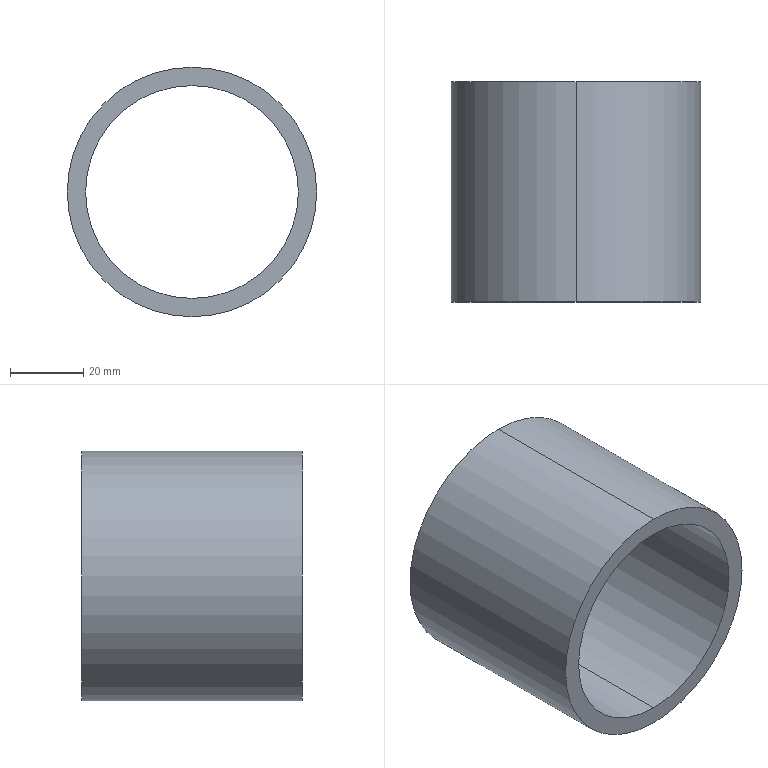Part | STEP file | outer cylinder block | 1 solid | 6 faces | box 68 x 60 x 68 mm | volume 59376 mm3 | cylinder 4 | plane 2 | commonest cylinder face diameters 58 x2 68 x2
STEP:
#1=CARTESIAN_POINT('',(0.,-30.,34.));
#2=VERTEX_POINT('',#1);
#3=CARTESIAN_POINT('',(0.,-30.,-34.));
#4=VERTEX_POINT('',#3);
#5=CARTESIAN_POINT('',(0.,-30.,0.));
#6=DIRECTION('',(0.,1.,0.));
#7=DIRECTION('',(0.,0.,1.));
#8=AXIS2_PLACEMENT_3D('',#5,#6,#7);
#9=CIRCLE('',#8,34.);
#10=EDGE_CURVE('',#2,#4,#9,.T.);
#11=ORIENTED_EDGE('',*,*,#10,.T.);
#12=CARTESIAN_POINT('',(0.,30.,-34.));
#13=VERTEX_POINT('',#12);
#14=CARTESIAN_POINT('',(0.,26.149,-34.));
#15=DIRECTION('',(0.,1.,0.));
#16=VECTOR('',#15,1000.);
#17=LINE('',#14,#16);
#18=EDGE_CURVE('',#4,#13,#17,.T.);
#19=ORIENTED_EDGE('',*,*,#18,.T.);
#20=CARTESIAN_POINT('',(0.,30.,34.));
#21=VERTEX_POINT('',#20);
#22=CARTESIAN_POINT('',(0.,30.,0.));
#23=DIRECTION('',(0.,1.,0.));
#24=DIRECTION('',(0.,0.,1.));
#25=AXIS2_PLACEMENT_3D('',#22,#23,#24);
#26=CIRCLE('',#25,34.);
#27=EDGE_CURVE('',#21,#13,#26,.T.);
#28=ORIENTED_EDGE('',*,*,#27,.F.);
#29=CARTESIAN_POINT('',(0.,26.149,34.));
#30=DIRECTION('',(0.,1.,0.));
#31=VECTOR('',#30,1000.);
#32=LINE('',#29,#31);
#33=EDGE_CURVE('',#2,#21,#32,.T.);
#34=ORIENTED_EDGE('',*,*,#33,.F.);
#35=EDGE_LOOP('',(#11,#19,#28,#34));
#36=FACE_OUTER_BOUND('',#35,.T.);
#37=CARTESIAN_POINT('',(0.,26.149,0.));
#38=DIRECTION('',(0.,1.,0.));
#39=DIRECTION('',(0.,0.,1.));
#40=AXIS2_PLACEMENT_3D('',#37,#38,#39);
#41=CYLINDRICAL_SURFACE('',#40,34.);
#42=ADVANCED_FACE('',(#36),#41,.T.);
#43=CARTESIAN_POINT('',(0.,-30.,-29.));
#44=VERTEX_POINT('',#43);
#45=CARTESIAN_POINT('',(0.,-30.,29.));
#46=VERTEX_POINT('',#45);
#47=CARTESIAN_POINT('',(0.,-30.,0.));
#48=DIRECTION('',(0.,1.,0.));
#49=DIRECTION('',(0.,0.,1.));
#50=AXIS2_PLACEMENT_3D('',#47,#48,#49);
#51=CIRCLE('',#50,29.);
#52=EDGE_CURVE('',#44,#46,#51,.T.);
#53=ORIENTED_EDGE('',*,*,#52,.F.);
#54=CARTESIAN_POINT('',(0.,30.,-29.));
#55=VERTEX_POINT('',#54);
#56=CARTESIAN_POINT('',(0.,26.149,-29.));
#57=DIRECTION('',(0.,1.,0.));
#58=VECTOR('',#57,1000.);
#59=LINE('',#56,#58);
#60=EDGE_CURVE('',#44,#55,#59,.T.);
#61=ORIENTED_EDGE('',*,*,#60,.T.);
#62=CARTESIAN_POINT('',(0.,30.,29.));
#63=VERTEX_POINT('',#62);
#64=CARTESIAN_POINT('',(0.,30.,0.));
#65=DIRECTION('',(0.,1.,0.));
#66=DIRECTION('',(0.,0.,1.));
#67=AXIS2_PLACEMENT_3D('',#64,#65,#66);
#68=CIRCLE('',#67,29.);
#69=EDGE_CURVE('',#55,#63,#68,.T.);
#70=ORIENTED_EDGE('',*,*,#69,.T.);
#71=CARTESIAN_POINT('',(0.,26.149,29.));
#72=DIRECTION('',(0.,1.,0.));
#73=VECTOR('',#72,1000.);
#74=LINE('',#71,#73);
#75=EDGE_CURVE('',#46,#63,#74,.T.);
#76=ORIENTED_EDGE('',*,*,#75,.F.);
#77=EDGE_LOOP('',(#53,#61,#70,#76));
#78=FACE_OUTER_BOUND('',#77,.T.);
#79=CARTESIAN_POINT('',(0.,26.149,0.));
#80=DIRECTION('',(0.,1.,0.));
#81=DIRECTION('',(0.,0.,1.));
#82=AXIS2_PLACEMENT_3D('',#79,#80,#81);
#83=CYLINDRICAL_SURFACE('',#82,29.);
#84=ADVANCED_FACE('',(#78),#83,.F.);
#85=ORIENTED_EDGE('',*,*,#60,.F.);
#86=CARTESIAN_POINT('',(0.,-30.,0.));
#87=DIRECTION('',(0.,1.,0.));
#88=DIRECTION('',(0.,0.,1.));
#89=AXIS2_PLACEMENT_3D('',#86,#87,#88);
#90=CIRCLE('',#89,29.);
#91=EDGE_CURVE('',#46,#44,#90,.T.);
#92=ORIENTED_EDGE('',*,*,#91,.F.);
#93=ORIENTED_EDGE('',*,*,#75,.T.);
#94=CARTESIAN_POINT('',(0.,30.,0.));
#95=DIRECTION('',(0.,1.,0.));
#96=DIRECTION('',(0.,0.,1.));
#97=AXIS2_PLACEMENT_3D('',#94,#95,#96);
#98=CIRCLE('',#97,29.);
#99=EDGE_CURVE('',#63,#55,#98,.T.);
#100=ORIENTED_EDGE('',*,*,#99,.T.);
#101=EDGE_LOOP('',(#85,#92,#93,#100));
#102=FACE_OUTER_BOUND('',#101,.T.);
#103=CARTESIAN_POINT('',(0.,26.149,0.));
#104=DIRECTION('',(0.,1.,0.));
#105=DIRECTION('',(0.,0.,1.));
#106=AXIS2_PLACEMENT_3D('',#103,#104,#105);
#107=CYLINDRICAL_SURFACE('',#106,29.);
#108=ADVANCED_FACE('',(#102),#107,.F.);
#109=ORIENTED_EDGE('',*,*,#27,.T.);
#110=CARTESIAN_POINT('',(0.,30.,0.));
#111=DIRECTION('',(0.,1.,0.));
#112=DIRECTION('',(0.,0.,1.));
#113=AXIS2_PLACEMENT_3D('',#110,#111,#112);
#114=CIRCLE('',#113,34.);
#115=EDGE_CURVE('',#13,#21,#114,.T.);
#116=ORIENTED_EDGE('',*,*,#115,.T.);
#117=EDGE_LOOP('',(#109,#116));
#118=FACE_OUTER_BOUND('',#117,.T.);
#119=ORIENTED_EDGE('',*,*,#99,.F.);
#120=ORIENTED_EDGE('',*,*,#69,.F.);
#121=EDGE_LOOP('',(#119,#120));
#122=FACE_BOUND('',#121,.T.);
#123=CARTESIAN_POINT('',(-34.,30.,0.));
#124=DIRECTION('',(0.,1.,0.));
#125=DIRECTION('',(0.,0.,1.));
#126=AXIS2_PLACEMENT_3D('',#123,#124,#125);
#127=PLANE('',#126);
#128=ADVANCED_FACE('',(#118,#122),#127,.T.);
#129=ORIENTED_EDGE('',*,*,#18,.F.);
#130=CARTESIAN_POINT('',(0.,-30.,0.));
#131=DIRECTION('',(0.,1.,0.));
#132=DIRECTION('',(0.,0.,1.));
#133=AXIS2_PLACEMENT_3D('',#130,#131,#132);
#134=CIRCLE('',#133,34.);
#135=EDGE_CURVE('',#4,#2,#134,.T.);
#136=ORIENTED_EDGE('',*,*,#135,.T.);
#137=ORIENTED_EDGE('',*,*,#33,.T.);
#138=ORIENTED_EDGE('',*,*,#115,.F.);
#139=EDGE_LOOP('',(#129,#136,#137,#138));
#140=FACE_OUTER_BOUND('',#139,.T.);
#141=CARTESIAN_POINT('',(0.,26.149,0.));
#142=DIRECTION('',(0.,1.,0.));
#143=DIRECTION('',(0.,0.,1.));
#144=AXIS2_PLACEMENT_3D('',#141,#142,#143);
#145=CYLINDRICAL_SURFACE('',#144,34.);
#146=ADVANCED_FACE('',(#140),#145,.T.);
#147=ORIENTED_EDGE('',*,*,#91,.T.);
#148=ORIENTED_EDGE('',*,*,#52,.T.);
#149=EDGE_LOOP('',(#147,#148));
#150=FACE_BOUND('',#149,.T.);
#151=ORIENTED_EDGE('',*,*,#10,.F.);
#152=ORIENTED_EDGE('',*,*,#135,.F.);
#153=EDGE_LOOP('',(#151,#152));
#154=FACE_OUTER_BOUND('',#153,.T.);
#155=CARTESIAN_POINT('',(-34.,-30.,0.));
#156=DIRECTION('',(0.,-1.,0.));
#157=DIRECTION('',(0.,0.,-1.));
#158=AXIS2_PLACEMENT_3D('',#155,#156,#157);
#159=PLANE('',#158);
#160=ADVANCED_FACE('',(#150,#154),#159,.T.);
#161=CLOSED_SHELL('',(#42,#84,#108,#128,#146,#160));
#162=MANIFOLD_SOLID_BREP('',#161);
#163=CARTESIAN_POINT('',(0.,0.,0.));
#164=DIRECTION('',(0.,0.,1.));
#165=DIRECTION('',(1.,0.,0.));
#166=AXIS2_PLACEMENT_3D('',#163,#164,#165);
#167=(LENGTH_UNIT()NAMED_UNIT(*)SI_UNIT(.MILLI.,.METRE.));
#168=UNCERTAINTY_MEASURE_WITH_UNIT(LENGTH_MEASURE(0.00001),#167,'','');
#169=(NAMED_UNIT(*)PLANE_ANGLE_UNIT()SI_UNIT($,.RADIAN.));
#170=(NAMED_UNIT(*)SI_UNIT($,.STERADIAN.)SOLID_ANGLE_UNIT());
#171=(GEOMETRIC_REPRESENTATION_CONTEXT(3)GLOBAL_UNCERTAINTY_ASSIGNED_CONTEXT((#168))GLOBAL_UNIT_ASSIGNED_CONTEXT((#167,#169,#170))REPRESENTATION_CONTEXT('',''));
#172=ADVANCED_BREP_SHAPE_REPRESENTATION('',(#162,#166),#171);